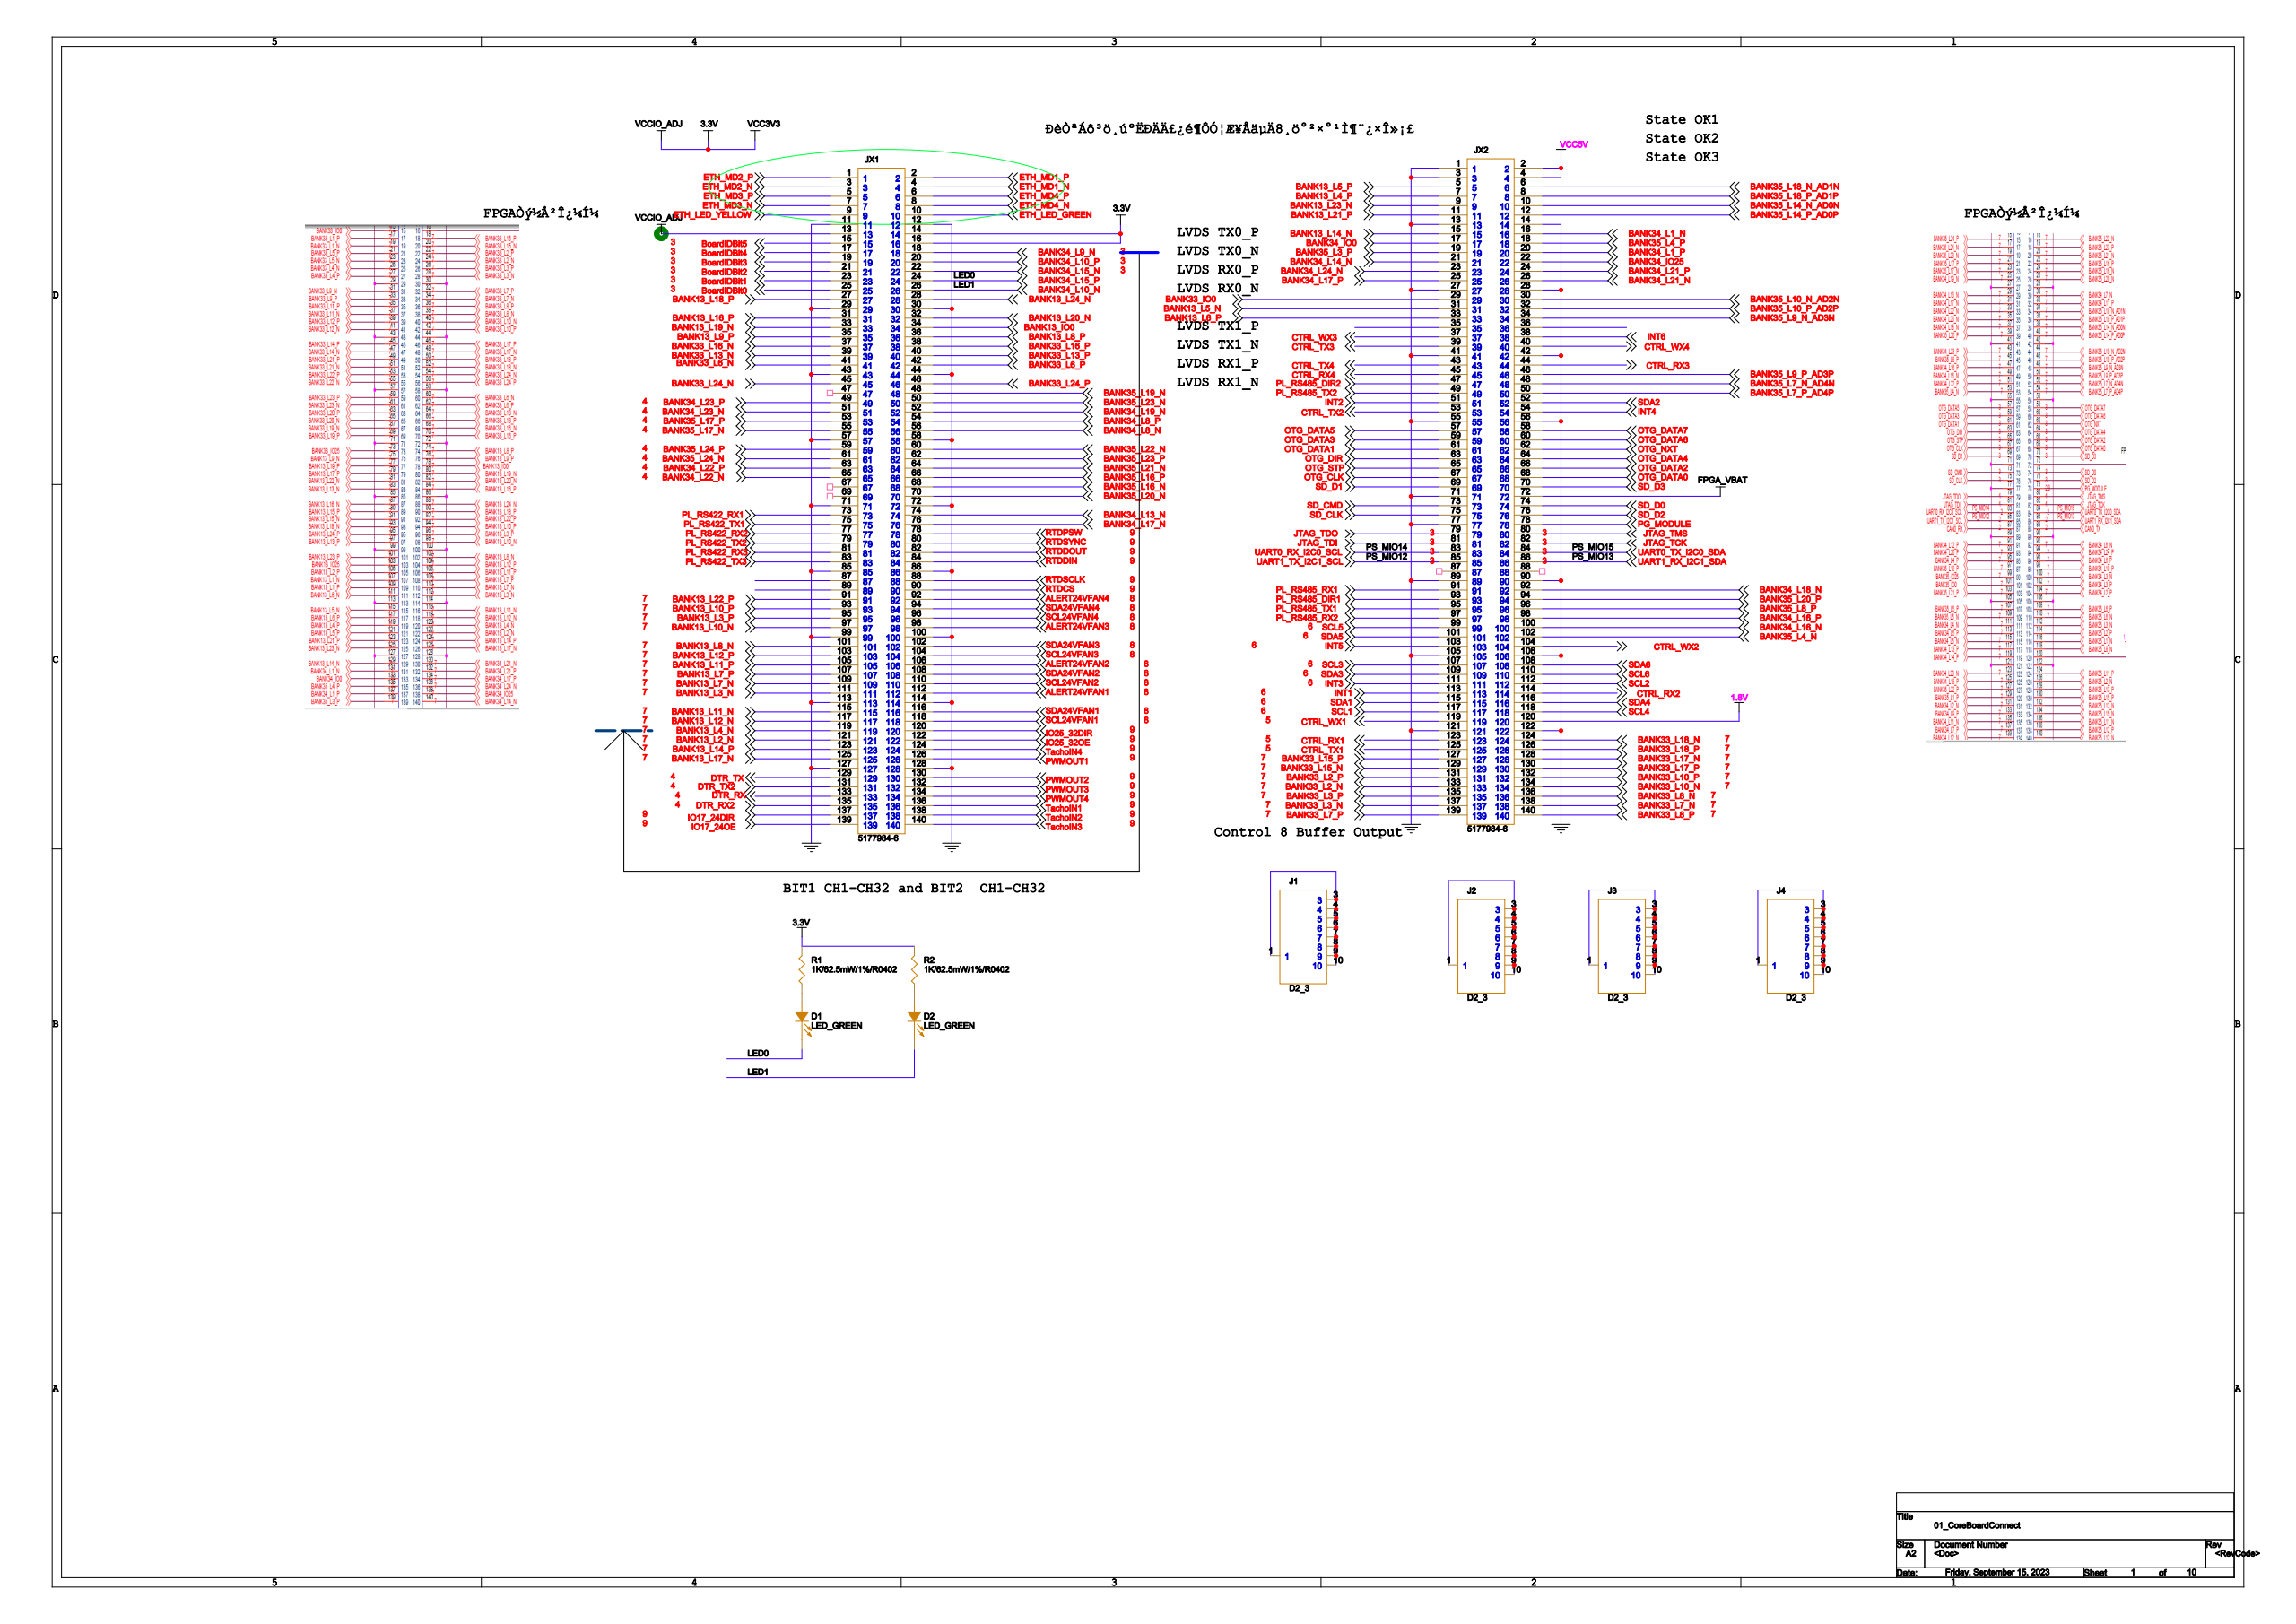Circuit board | Cadence Allegro | 634 parts | 645 nets | one sheet of the schematic
Parts on this sheet (reference | value | footprint):
D1 | LED_GREEN | LED0805
D2 | LED_GREEN | LED0805
J1 | D2_3 | D2_3
J2 | D2_3 | D2_3
J3 | D2_3 | D2_3
J4 | D2_3 | D2_3
JX1 | 5177984-6 | 5177983-6
JX2 | 5177984-6 | 5177983-6
R1 | 1K/62.5mW/1%/R0402 | 0402
R2 | 1K/62.5mW/1%/R0402 | 0402
Nets of these parts (net: part-pin ...):
ETH_MD2_P: JX1-1
ETH_LED_GREEN: JX1-10
BANK13_L8_N: JX1-101
SDA24VFAN3: JX1-102
BANK13_L12_P: JX1-103
SCL24VFAN3: JX1-104
BANK13_L11_P: JX1-105
ALERT24VFAN2: JX1-106
BANK13_L7_P: JX1-107
SDA24VFAN2: JX1-108
BANK13_L7_N: JX1-109
SCL24VFAN2: JX1-110
BANK13_L3_N: JX1-111
ALERT24VFAN1: JX1-112
BANK13_L11_N: JX1-115
SDA24VFAN1: JX1-116
BANK13_L12_N: JX1-117
SCL24VFAN1: JX1-118
BANK13_L4_N: JX1-119
IO25_32DIR: JX1-120
BANK13_L2_N: JX1-121
IO25_32OE: JX1-122
BANK13_L14_P: JX1-123
BANK13_L17_N: JX1-125
PWMOUT1: JX1-126
DTR_TX: JX1-129
3.3V: R1-2 R2-2 JX1-13 JX1-14 JX1-16
PWMOUT2: JX1-130
DTR_TX2: JX1-131
PWMOUT3: JX1-132
DTR_RX: JX1-133
PWMOUT4: JX1-134
DTR_RX2: JX1-135
IO17_24DIR: JX1-137
IO17_24OE: JX1-139
BANK34_L9_N: JX1-18
ETH_MD1_P: JX1-2
BANK34_L10_P: JX1-20
BANK34_L15_N: JX1-22
BANK34_L15_P: D1-2 JX1-24
BANK34_L10_N: D2-2 JX1-26
BANK13_L18_P: JX1-27
BANK13_L24_N: JX1-28
ETH_MD2_N: JX1-3
BANK13_L16_P: JX1-31
BANK13_L20_N: JX1-32
BANK13_L19_N: JX1-33
BANK13_IO0: JX1-34
BANK13_L9_P: JX1-35
BANK13_L8_P: JX1-36
BANK33_L16_N: JX1-37
BANK33_L16_P: JX1-38
BANK33_L13_N: JX1-39
ETH_MD1_N: JX1-4
BANK33_L13_P: JX1-40
BANK33_L6_N: JX1-41
BANK33_L6_P: JX1-42
BANK33_L24_N: JX1-45
BANK33_L24_P: JX1-46
BANK35_L19_N: JX1-48
BANK34_L23_P: JX1-49
ETH_MD3_P: JX1-5
BANK35_L23_N: JX1-50
BANK34_L23_N: JX1-51
BANK34_L19_N: JX1-52
BANK35_L17_P: JX1-53
BANK34_L8_P: JX1-54
BANK35_L17_N: JX1-55
BANK34_L8_N: JX1-56
BANK35_L24_P: JX1-59
ETH_MD4_P: JX1-6
BANK35_L22_N: JX1-60
BANK35_L24_N: JX1-61
BANK35_L23_P: JX1-62
BANK34_L22_P: JX1-63
BANK35_L21_N: JX1-64
BANK34_L22_N: JX1-65
BANK35_L16_P: JX1-66
BANK35_L16_N: JX1-68
ETH_MD3_N: JX1-7
BANK35_L20_N: JX1-70
PL_RS422_RX1: JX1-73
BANK34_L13_N: JX1-74
PL_RS422_TX1: JX1-75
BANK34_L17_N: JX1-76
PL_RS422_RX2: JX1-77
RTDPSW: JX1-78
PL_RS422_TX2: JX1-79
ETH_MD4_N: JX1-8
RTDSYNC: JX1-80
PL_RS422_RX3: JX1-81
RTDDOUT: JX1-82
PL_RS422_TX3: JX1-83
RTDDIN: JX1-84
RTDSCLK: JX1-88
ETH_LED_YELLOW: JX1-9
RTDCS: JX1-90
BANK13_L22_P: JX1-91
ALERT24VFAN4: JX1-92
BANK13_L10_P: JX1-93
SDA24VFAN4: JX1-94
BANK13_L3_P: JX1-95
SCL24VFAN4: JX1-96
BANK13_L10_N: JX1-97
ALERT24VFAN3: JX1-98
BANK35_L14_N_AD0N: JX2-10
BANK34_L16_N: JX2-100
SDA5: JX2-101
BANK35_L4_N: JX2-102
INT5: JX2-103
CTRL_WX2: JX2-104
SCL3: JX2-107
SDA6: JX2-108
SDA3: JX2-109
BANK13_L21_P: JX2-11
SCL6: JX2-110
INT3: JX2-111
SCL2: JX2-112
INT1: JX2-113
CTRL_RX2: JX2-114
SDA1: JX2-115
SDA4: JX2-116
SCL1: JX2-117
SCL4: JX2-118
CTRL_WX1: JX2-119
BANK35_L14_P_AD0P: JX2-12
1.8V: JX2-120
CTRL_RX1: JX2-123
BANK33_L18_N: JX2-124
CTRL_TX1: JX2-125
BANK33_L18_P: JX2-126
BANK33_L15_P: JX2-127
BANK33_L17_N: JX2-128
BANK33_L15_N: JX2-129
BANK33_L17_P: JX2-130
BANK33_L2_P: JX2-131
BANK33_L10_P: JX2-132
BANK33_L2_N: JX2-133
BANK33_L10_N: JX2-134
BANK33_L3_P: JX2-135
BANK33_L8_N: JX2-136
BANK33_L3_N: JX2-137
BANK33_L7_N: JX2-138
BANK33_L7_P: JX2-139
BANK33_L8_P: JX2-140
BANK13_L14_N: JX2-15
BANK34_L1_N: JX2-16
BANK34_IO0: JX2-17
BANK35_L4_P: JX2-18
BANK35_L3_P: JX2-19
VCC5V: JX2-2 JX2-4
BANK34_L1_P: JX2-20
BANK34_L14_N: JX2-21
BANK34_IO25: JX2-22
BANK34_L24_N: JX2-23
BANK34_L21_P: JX2-24
BANK34_L17_P: JX2-25
BANK34_L21_N: JX2-26
BANK33_IO0: JX2-29
BANK35_L10_N_AD2N: JX2-30
BANK13_L5_N: JX2-31
BANK35_L10_P_AD2P: JX2-32
BANK13_L6_P: JX2-33
BANK35_L9_N_AD3N: JX2-34
CTRL_WX3: JX2-37
INT6: JX2-38
CTRL_TX3: JX2-39
CTRL_WX4: JX2-40
CTRL_TX4: JX2-43
CTRL_RX3: JX2-44
CTRL_RX4: JX2-45
BANK35_L9_P_AD3P: JX2-46
PL_RS485_DIR2: JX2-47
BANK35_L7_N_AD4N: JX2-48
PL_RS485_TX2: JX2-49
BANK13_L5_P: JX2-5
BANK35_L7_P_AD4P: JX2-50
INT2: JX2-51
SDA2: JX2-52
CTRL_TX2: JX2-53
INT4: JX2-54
OTG_DATA5: JX2-57
OTG_DATA7: JX2-58
OTG_DATA3: JX2-59
BANK35_L18_N_AD1N: JX2-6
OTG_DATA6: JX2-60
OTG_DATA1: JX2-61
OTG_NXT: JX2-62
OTG_DIR: JX2-63
OTG_DATA4: JX2-64
OTG_STP: JX2-65
OTG_DATA2: JX2-66
OTG_CLK: JX2-67
OTG_DATA0: JX2-68
SD_D1: JX2-69
BANK13_L4_P: JX2-7
SD_D3: JX2-70
FPGA_VBAT: JX2-72
SD_CMD: JX2-73
SD_D0: JX2-74
SD_CLK: JX2-75
SD_D2: JX2-76
PG_MODULE: JX2-78
JTAG_TDO: JX2-79
BANK35_L18_P_AD1P: JX2-8
JTAG_TMS: JX2-80
JTAG_TDI: JX2-81
JTAG_TCK: JX2-82
UART0_RX_I2C0_SCL: JX2-83
UART0_TX_I2C0_SDA: JX2-84
UART1_TX_I2C1_SCL: JX2-85
UART1_RX_I2C1_SDA: JX2-86
BANK13_L23_N: JX2-9
PL_RS485_RX1: JX2-91
BANK34_L18_N: JX2-92
PL_RS485_DIR1: JX2-93
BANK35_L20_P: JX2-94
PL_RS485_TX1: JX2-95
BANK35_L8_P: JX2-96
PL_RS485_RX2: JX2-97
BANK34_L16_P: JX2-98
SCL5: JX2-99
N231084320: D1-1 R1-1
N231087860: D2-1 R2-1
N23884939: J1-1 J1-3 J1-4 J1-5 J1-6 J1-7 J1-8 J1-9 J1-10
N23884945: J2-1 J2-3 J2-4 J2-5 J2-6 J2-7 J2-8 J2-9 J2-10
N23884981: J3-1 J3-3 J3-4 J3-5 J3-6 J3-7 J3-8 J3-9 J3-10
N23884987: J4-1 J4-3 J4-4 J4-5 J4-6 J4-7 J4-8 J4-9 J4-10